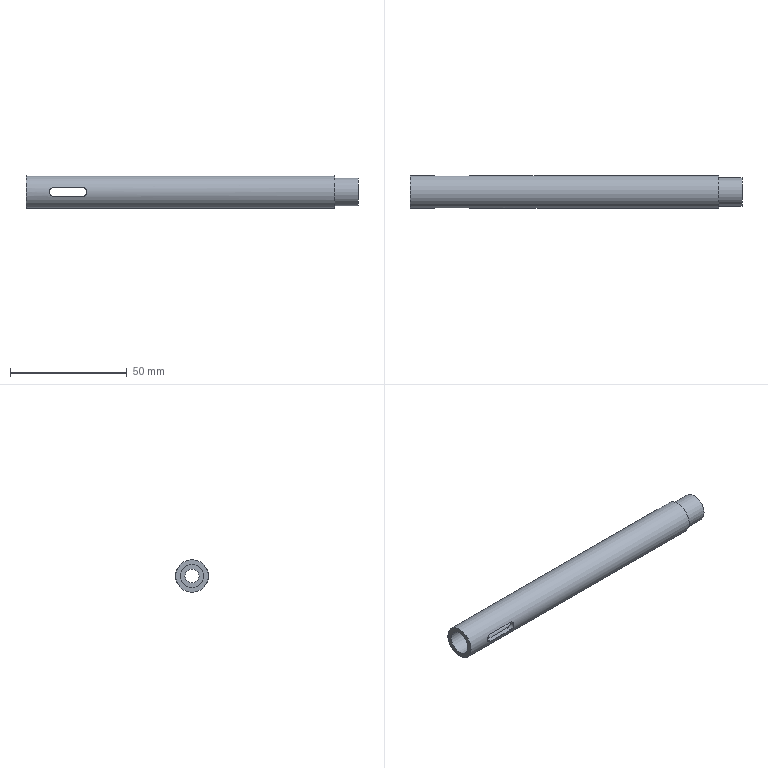Part | STEP file | 1-23.2 | 1 solid | 16 faces | box 142 x 14 x 14 mm | volume 14676 mm3 | cylinder 8 | plane 8 | commonest cylinder face diameters 4 x4 6 x1 10 x1 12 x1 14 x1